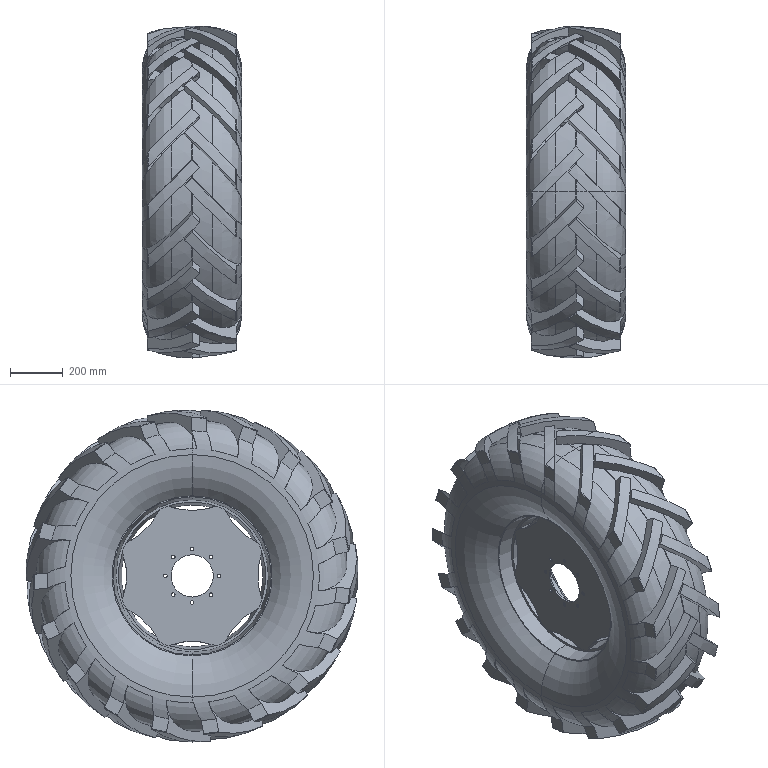Part | SolidWorks | features CirPattern 2, ICE 2, RevCut 2, Revolution 2, Fillet 1, MoveFace 1 | 1 solid | 430 faces | box 378 x 1264 x 1263 mm | volume 294316338 mm3 | torus 213 | plane 158 | cylinder 36 | cone 23 | commonest cylinder face diameters 539 x18 14 x16 161 x2